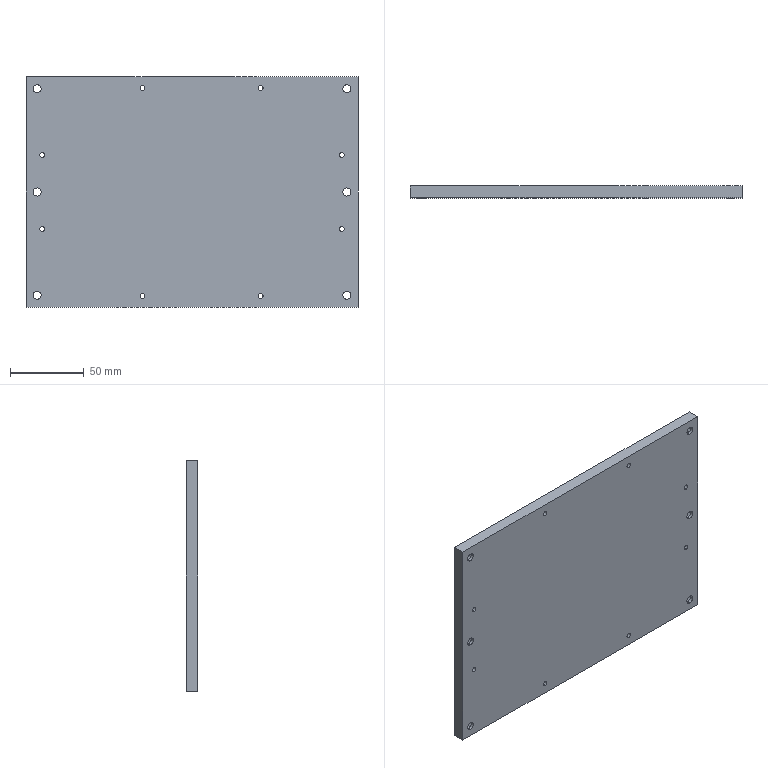Part | SolidWorks | features 3DProfileFeature 3, HoleWzd 3, MirrorPattern 3, Extrusion 1 | 1 solid | 52 faces | box 225 x 8 x 156 mm | volume 277140 mm3 | cylinder 40 | plane 12 | commonest cylinder face diameters 3.3 x16 5.5 x12 10 x12